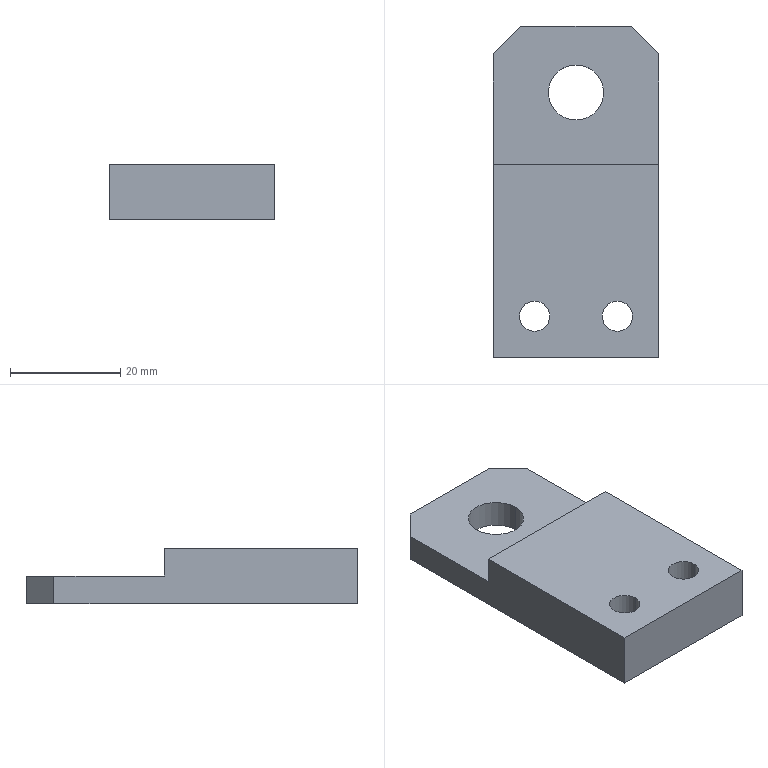Part | STEP file | slingshot displacement cylinder seat | 1 solid | 16 faces | box 30 x 60 x 10 mm | volume 13257 mm3 | plane 10 | cylinder 6 | commonest cylinder face diameters 5.5 x4 10 x2
STEP:
#1=CARTESIAN_POINT('',(0.,0.,0.));
#2=DIRECTION('',(0.,0.,1.));
#3=DIRECTION('',(1.,0.,0.));
#4=AXIS2_PLACEMENT_3D('',#1,#2,#3);
#5=CARTESIAN_POINT('',(-18.899,-2.623,0.));
#6=VERTEX_POINT('',#5);
#7=CARTESIAN_POINT('',(-18.899,-2.623,10.));
#8=VERTEX_POINT('',#7);
#9=CARTESIAN_POINT('',(-18.899,-2.623,0.));
#10=DIRECTION('',(0.,0.,1.));
#11=VECTOR('',#10,1.);
#12=LINE('',#9,#11);
#13=CARTESIAN_POINT('',(-21.649,-2.623,0.));
#14=DIRECTION('',(0.,0.,1.));
#15=DIRECTION('',(1.,0.,0.));
#16=AXIS2_PLACEMENT_3D('',#13,#14,#15);
#17=CYLINDRICAL_SURFACE('',#16,2.75);
#18=CARTESIAN_POINT('',(6.283,0.));
#19=DIRECTION('',(0.,1.));
#20=VECTOR('',#19,1.);
#21=LINE('',#18,#20);
#22=(GEOMETRIC_REPRESENTATION_CONTEXT(2)PARAMETRIC_REPRESENTATION_CONTEXT()REPRESENTATION_CONTEXT('',''));
#23=DEFINITIONAL_REPRESENTATION('',(#21),#22);
#24=PCURVE('',#17,#23);
#25=CARTESIAN_POINT('',(-21.649,-2.623,0.));
#26=DIRECTION('',(0.,0.,1.));
#27=DIRECTION('',(1.,0.,0.));
#28=AXIS2_PLACEMENT_3D('',#25,#26,#27);
#29=CYLINDRICAL_SURFACE('',#28,2.75);
#30=CARTESIAN_POINT('',(0.,0.));
#31=DIRECTION('',(0.,1.));
#32=VECTOR('',#31,1.);
#33=LINE('',#30,#32);
#34=(GEOMETRIC_REPRESENTATION_CONTEXT(2)PARAMETRIC_REPRESENTATION_CONTEXT()REPRESENTATION_CONTEXT('',''));
#35=DEFINITIONAL_REPRESENTATION('',(#33),#34);
#36=PCURVE('',#29,#35);
#37=SURFACE_CURVE('',#12,(#24,#36),.PCURVE_S1.);
#38=EDGE_CURVE('',#6,#8,#37,.T.);
#39=ORIENTED_EDGE('',*,*,#38,.T.);
#40=CARTESIAN_POINT('',(-24.399,-2.623,10.));
#41=VERTEX_POINT('',#40);
#42=CARTESIAN_POINT('',(-21.649,-2.623,10.));
#43=DIRECTION('',(0.,0.,1.));
#44=DIRECTION('',(1.,0.,0.));
#45=AXIS2_PLACEMENT_3D('',#42,#43,#44);
#46=CIRCLE('',#45,2.75);
#47=CARTESIAN_POINT('',(0.,10.));
#48=DIRECTION('',(1.,0.));
#49=VECTOR('',#48,1.);
#50=LINE('',#47,#49);
#51=(GEOMETRIC_REPRESENTATION_CONTEXT(2)PARAMETRIC_REPRESENTATION_CONTEXT()REPRESENTATION_CONTEXT('',''));
#52=DEFINITIONAL_REPRESENTATION('',(#50),#51);
#53=PCURVE('',#17,#52);
#54=CARTESIAN_POINT('',(-29.149,-10.123,10.));
#55=DIRECTION('',(0.,0.,1.));
#56=DIRECTION('',(1.,0.,0.));
#57=AXIS2_PLACEMENT_3D('',#54,#55,#56);
#58=PLANE('',#57);
#59=CARTESIAN_POINT('',(7.5,7.5));
#60=DIRECTION('',(1.,0.));
#61=AXIS2_PLACEMENT_2D('',#59,#60);
#62=CIRCLE('',#61,2.75);
#63=(GEOMETRIC_REPRESENTATION_CONTEXT(2)PARAMETRIC_REPRESENTATION_CONTEXT()REPRESENTATION_CONTEXT('',''));
#64=DEFINITIONAL_REPRESENTATION('',(#62),#63);
#65=PCURVE('',#58,#64);
#66=SURFACE_CURVE('',#46,(#53,#65),.PCURVE_S1.);
#67=EDGE_CURVE('',#41,#8,#66,.T.);
#68=ORIENTED_EDGE('',*,*,#67,.F.);
#69=CARTESIAN_POINT('',(-24.399,-2.623,0.));
#70=VERTEX_POINT('',#69);
#71=CARTESIAN_POINT('',(-24.399,-2.623,0.));
#72=DIRECTION('',(0.,0.,1.));
#73=VECTOR('',#72,1.);
#74=LINE('',#71,#73);
#75=CARTESIAN_POINT('',(3.142,0.));
#76=DIRECTION('',(0.,1.));
#77=VECTOR('',#76,1.);
#78=LINE('',#75,#77);
#79=(GEOMETRIC_REPRESENTATION_CONTEXT(2)PARAMETRIC_REPRESENTATION_CONTEXT()REPRESENTATION_CONTEXT('',''));
#80=DEFINITIONAL_REPRESENTATION('',(#78),#79);
#81=PCURVE('',#17,#80);
#82=CARTESIAN_POINT('',(3.142,0.));
#83=DIRECTION('',(0.,1.));
#84=VECTOR('',#83,1.);
#85=LINE('',#82,#84);
#86=(GEOMETRIC_REPRESENTATION_CONTEXT(2)PARAMETRIC_REPRESENTATION_CONTEXT()REPRESENTATION_CONTEXT('',''));
#87=DEFINITIONAL_REPRESENTATION('',(#85),#86);
#88=PCURVE('',#29,#87);
#89=SURFACE_CURVE('',#74,(#81,#88),.PCURVE_S1.);
#90=EDGE_CURVE('',#70,#41,#89,.T.);
#91=ORIENTED_EDGE('',*,*,#90,.F.);
#92=CARTESIAN_POINT('',(-21.649,-2.623,0.));
#93=DIRECTION('',(0.,0.,1.));
#94=DIRECTION('',(1.,0.,0.));
#95=AXIS2_PLACEMENT_3D('',#92,#93,#94);
#96=CIRCLE('',#95,2.75);
#97=CARTESIAN_POINT('',(0.,0.));
#98=DIRECTION('',(1.,0.));
#99=VECTOR('',#98,1.);
#100=LINE('',#97,#99);
#101=(GEOMETRIC_REPRESENTATION_CONTEXT(2)PARAMETRIC_REPRESENTATION_CONTEXT()REPRESENTATION_CONTEXT('',''));
#102=DEFINITIONAL_REPRESENTATION('',(#100),#101);
#103=PCURVE('',#17,#102);
#104=CARTESIAN_POINT('',(-29.149,-10.123,0.));
#105=DIRECTION('',(0.,0.,1.));
#106=DIRECTION('',(1.,0.,0.));
#107=AXIS2_PLACEMENT_3D('',#104,#105,#106);
#108=PLANE('',#107);
#109=CARTESIAN_POINT('',(7.5,7.5));
#110=DIRECTION('',(1.,0.));
#111=AXIS2_PLACEMENT_2D('',#109,#110);
#112=CIRCLE('',#111,2.75);
#113=(GEOMETRIC_REPRESENTATION_CONTEXT(2)PARAMETRIC_REPRESENTATION_CONTEXT()REPRESENTATION_CONTEXT('',''));
#114=DEFINITIONAL_REPRESENTATION('',(#112),#113);
#115=PCURVE('',#108,#114);
#116=SURFACE_CURVE('',#96,(#103,#115),.PCURVE_S1.);
#117=EDGE_CURVE('',#70,#6,#116,.T.);
#118=ORIENTED_EDGE('',*,*,#117,.T.);
#119=EDGE_LOOP('',(#39,#68,#91,#118));
#120=FACE_BOUND('',#119,.F.);
#121=ADVANCED_FACE('',(#120),#17,.F.);
#122=CARTESIAN_POINT('',(-3.899,-2.623,0.));
#123=VERTEX_POINT('',#122);
#124=CARTESIAN_POINT('',(-3.899,-2.623,10.));
#125=VERTEX_POINT('',#124);
#126=CARTESIAN_POINT('',(-3.899,-2.623,0.));
#127=DIRECTION('',(0.,0.,1.));
#128=VECTOR('',#127,1.);
#129=LINE('',#126,#128);
#130=CARTESIAN_POINT('',(-6.649,-2.623,0.));
#131=DIRECTION('',(0.,0.,1.));
#132=DIRECTION('',(1.,0.,0.));
#133=AXIS2_PLACEMENT_3D('',#130,#131,#132);
#134=CYLINDRICAL_SURFACE('',#133,2.75);
#135=CARTESIAN_POINT('',(6.283,0.));
#136=DIRECTION('',(0.,1.));
#137=VECTOR('',#136,1.);
#138=LINE('',#135,#137);
#139=(GEOMETRIC_REPRESENTATION_CONTEXT(2)PARAMETRIC_REPRESENTATION_CONTEXT()REPRESENTATION_CONTEXT('',''));
#140=DEFINITIONAL_REPRESENTATION('',(#138),#139);
#141=PCURVE('',#134,#140);
#142=CARTESIAN_POINT('',(-6.649,-2.623,0.));
#143=DIRECTION('',(0.,0.,1.));
#144=DIRECTION('',(1.,0.,0.));
#145=AXIS2_PLACEMENT_3D('',#142,#143,#144);
#146=CYLINDRICAL_SURFACE('',#145,2.75);
#147=CARTESIAN_POINT('',(0.,0.));
#148=DIRECTION('',(0.,1.));
#149=VECTOR('',#148,1.);
#150=LINE('',#147,#149);
#151=(GEOMETRIC_REPRESENTATION_CONTEXT(2)PARAMETRIC_REPRESENTATION_CONTEXT()REPRESENTATION_CONTEXT('',''));
#152=DEFINITIONAL_REPRESENTATION('',(#150),#151);
#153=PCURVE('',#146,#152);
#154=SURFACE_CURVE('',#129,(#141,#153),.PCURVE_S1.);
#155=EDGE_CURVE('',#123,#125,#154,.T.);
#156=ORIENTED_EDGE('',*,*,#155,.T.);
#157=CARTESIAN_POINT('',(-9.399,-2.623,10.));
#158=VERTEX_POINT('',#157);
#159=CARTESIAN_POINT('',(-6.649,-2.623,10.));
#160=DIRECTION('',(0.,0.,1.));
#161=DIRECTION('',(1.,0.,0.));
#162=AXIS2_PLACEMENT_3D('',#159,#160,#161);
#163=CIRCLE('',#162,2.75);
#164=CARTESIAN_POINT('',(0.,10.));
#165=DIRECTION('',(1.,0.));
#166=VECTOR('',#165,1.);
#167=LINE('',#164,#166);
#168=(GEOMETRIC_REPRESENTATION_CONTEXT(2)PARAMETRIC_REPRESENTATION_CONTEXT()REPRESENTATION_CONTEXT('',''));
#169=DEFINITIONAL_REPRESENTATION('',(#167),#168);
#170=PCURVE('',#134,#169);
#171=CARTESIAN_POINT('',(22.5,7.5));
#172=DIRECTION('',(1.,0.));
#173=AXIS2_PLACEMENT_2D('',#171,#172);
#174=CIRCLE('',#173,2.75);
#175=(GEOMETRIC_REPRESENTATION_CONTEXT(2)PARAMETRIC_REPRESENTATION_CONTEXT()REPRESENTATION_CONTEXT('',''));
#176=DEFINITIONAL_REPRESENTATION('',(#174),#175);
#177=PCURVE('',#58,#176);
#178=SURFACE_CURVE('',#163,(#170,#177),.PCURVE_S1.);
#179=EDGE_CURVE('',#158,#125,#178,.T.);
#180=ORIENTED_EDGE('',*,*,#179,.F.);
#181=CARTESIAN_POINT('',(-9.399,-2.623,0.));
#182=VERTEX_POINT('',#181);
#183=CARTESIAN_POINT('',(-9.399,-2.623,0.));
#184=DIRECTION('',(0.,0.,1.));
#185=VECTOR('',#184,1.);
#186=LINE('',#183,#185);
#187=CARTESIAN_POINT('',(3.142,0.));
#188=DIRECTION('',(0.,1.));
#189=VECTOR('',#188,1.);
#190=LINE('',#187,#189);
#191=(GEOMETRIC_REPRESENTATION_CONTEXT(2)PARAMETRIC_REPRESENTATION_CONTEXT()REPRESENTATION_CONTEXT('',''));
#192=DEFINITIONAL_REPRESENTATION('',(#190),#191);
#193=PCURVE('',#134,#192);
#194=CARTESIAN_POINT('',(3.142,0.));
#195=DIRECTION('',(0.,1.));
#196=VECTOR('',#195,1.);
#197=LINE('',#194,#196);
#198=(GEOMETRIC_REPRESENTATION_CONTEXT(2)PARAMETRIC_REPRESENTATION_CONTEXT()REPRESENTATION_CONTEXT('',''));
#199=DEFINITIONAL_REPRESENTATION('',(#197),#198);
#200=PCURVE('',#146,#199);
#201=SURFACE_CURVE('',#186,(#193,#200),.PCURVE_S1.);
#202=EDGE_CURVE('',#182,#158,#201,.T.);
#203=ORIENTED_EDGE('',*,*,#202,.F.);
#204=CARTESIAN_POINT('',(-6.649,-2.623,0.));
#205=DIRECTION('',(0.,0.,1.));
#206=DIRECTION('',(1.,0.,0.));
#207=AXIS2_PLACEMENT_3D('',#204,#205,#206);
#208=CIRCLE('',#207,2.75);
#209=CARTESIAN_POINT('',(0.,0.));
#210=DIRECTION('',(1.,0.));
#211=VECTOR('',#210,1.);
#212=LINE('',#209,#211);
#213=(GEOMETRIC_REPRESENTATION_CONTEXT(2)PARAMETRIC_REPRESENTATION_CONTEXT()REPRESENTATION_CONTEXT('',''));
#214=DEFINITIONAL_REPRESENTATION('',(#212),#213);
#215=PCURVE('',#134,#214);
#216=CARTESIAN_POINT('',(22.5,7.5));
#217=DIRECTION('',(1.,0.));
#218=AXIS2_PLACEMENT_2D('',#216,#217);
#219=CIRCLE('',#218,2.75);
#220=(GEOMETRIC_REPRESENTATION_CONTEXT(2)PARAMETRIC_REPRESENTATION_CONTEXT()REPRESENTATION_CONTEXT('',''));
#221=DEFINITIONAL_REPRESENTATION('',(#219),#220);
#222=PCURVE('',#108,#221);
#223=SURFACE_CURVE('',#208,(#215,#222),.PCURVE_S1.);
#224=EDGE_CURVE('',#182,#123,#223,.T.);
#225=ORIENTED_EDGE('',*,*,#224,.T.);
#226=EDGE_LOOP('',(#156,#180,#203,#225));
#227=FACE_BOUND('',#226,.F.);
#228=ADVANCED_FACE('',(#227),#134,.F.);
#229=CARTESIAN_POINT('',(-19.149,37.877,5.));
#230=VERTEX_POINT('',#229);
#231=CARTESIAN_POINT('',(-19.149,37.877,0.));
#232=VERTEX_POINT('',#231);
#233=CARTESIAN_POINT('',(-19.149,37.877,10.));
#234=DIRECTION('',(0.,0.,-1.));
#235=VECTOR('',#234,1.);
#236=LINE('',#233,#235);
#237=CARTESIAN_POINT('',(-14.149,37.877,10.));
#238=DIRECTION('',(0.,0.,-1.));
#239=DIRECTION('',(-1.,0.,0.));
#240=AXIS2_PLACEMENT_3D('',#237,#238,#239);
#241=CYLINDRICAL_SURFACE('',#240,5.);
#242=CARTESIAN_POINT('',(6.283,0.));
#243=DIRECTION('',(0.,1.));
#244=VECTOR('',#243,1.);
#245=LINE('',#242,#244);
#246=(GEOMETRIC_REPRESENTATION_CONTEXT(2)PARAMETRIC_REPRESENTATION_CONTEXT()REPRESENTATION_CONTEXT('',''));
#247=DEFINITIONAL_REPRESENTATION('',(#245),#246);
#248=PCURVE('',#241,#247);
#249=CARTESIAN_POINT('',(-14.149,37.877,10.));
#250=DIRECTION('',(0.,0.,-1.));
#251=DIRECTION('',(-1.,0.,0.));
#252=AXIS2_PLACEMENT_3D('',#249,#250,#251);
#253=CYLINDRICAL_SURFACE('',#252,5.);
#254=CARTESIAN_POINT('',(0.,0.));
#255=DIRECTION('',(0.,1.));
#256=VECTOR('',#255,1.);
#257=LINE('',#254,#256);
#258=(GEOMETRIC_REPRESENTATION_CONTEXT(2)PARAMETRIC_REPRESENTATION_CONTEXT()REPRESENTATION_CONTEXT('',''));
#259=DEFINITIONAL_REPRESENTATION('',(#257),#258);
#260=PCURVE('',#253,#259);
#261=SURFACE_CURVE('',#236,(#248,#260),.PCURVE_S1.);
#262=EDGE_CURVE('',#230,#232,#261,.T.);
#263=ORIENTED_EDGE('',*,*,#262,.T.);
#264=CARTESIAN_POINT('',(-9.149,37.877,0.));
#265=VERTEX_POINT('',#264);
#266=CARTESIAN_POINT('',(-14.149,37.877,0.));
#267=DIRECTION('',(0.,0.,1.));
#268=DIRECTION('',(1.,0.,0.));
#269=AXIS2_PLACEMENT_3D('',#266,#267,#268);
#270=CIRCLE('',#269,5.);
#271=CARTESIAN_POINT('',(9.425,10.));
#272=DIRECTION('',(-1.,0.));
#273=VECTOR('',#272,1.);
#274=LINE('',#271,#273);
#275=(GEOMETRIC_REPRESENTATION_CONTEXT(2)PARAMETRIC_REPRESENTATION_CONTEXT()REPRESENTATION_CONTEXT('',''));
#276=DEFINITIONAL_REPRESENTATION('',(#274),#275);
#277=PCURVE('',#241,#276);
#278=CARTESIAN_POINT('',(15.,48.));
#279=DIRECTION('',(1.,0.));
#280=AXIS2_PLACEMENT_2D('',#278,#279);
#281=CIRCLE('',#280,5.);
#282=(GEOMETRIC_REPRESENTATION_CONTEXT(2)PARAMETRIC_REPRESENTATION_CONTEXT()REPRESENTATION_CONTEXT('',''));
#283=DEFINITIONAL_REPRESENTATION('',(#281),#282);
#284=PCURVE('',#108,#283);
#285=SURFACE_CURVE('',#270,(#277,#284),.PCURVE_S1.);
#286=EDGE_CURVE('',#232,#265,#285,.T.);
#287=ORIENTED_EDGE('',*,*,#286,.T.);
#288=CARTESIAN_POINT('',(-9.149,37.877,5.));
#289=VERTEX_POINT('',#288);
#290=CARTESIAN_POINT('',(-9.149,37.877,10.));
#291=DIRECTION('',(0.,0.,-1.));
#292=VECTOR('',#291,1.);
#293=LINE('',#290,#292);
#294=CARTESIAN_POINT('',(3.142,0.));
#295=DIRECTION('',(0.,1.));
#296=VECTOR('',#295,1.);
#297=LINE('',#294,#296);
#298=(GEOMETRIC_REPRESENTATION_CONTEXT(2)PARAMETRIC_REPRESENTATION_CONTEXT()REPRESENTATION_CONTEXT('',''));
#299=DEFINITIONAL_REPRESENTATION('',(#297),#298);
#300=PCURVE('',#241,#299);
#301=CARTESIAN_POINT('',(3.142,0.));
#302=DIRECTION('',(0.,1.));
#303=VECTOR('',#302,1.);
#304=LINE('',#301,#303);
#305=(GEOMETRIC_REPRESENTATION_CONTEXT(2)PARAMETRIC_REPRESENTATION_CONTEXT()REPRESENTATION_CONTEXT('',''));
#306=DEFINITIONAL_REPRESENTATION('',(#304),#305);
#307=PCURVE('',#253,#306);
#308=SURFACE_CURVE('',#293,(#300,#307),.PCURVE_S1.);
#309=EDGE_CURVE('',#289,#265,#308,.T.);
#310=ORIENTED_EDGE('',*,*,#309,.F.);
#311=CARTESIAN_POINT('',(-14.149,37.877,5.));
#312=DIRECTION('',(0.,0.,1.));
#313=DIRECTION('',(1.,0.,0.));
#314=AXIS2_PLACEMENT_3D('',#311,#312,#313);
#315=CIRCLE('',#314,5.);
#316=CARTESIAN_POINT('',(9.425,5.));
#317=DIRECTION('',(-1.,0.));
#318=VECTOR('',#317,1.);
#319=LINE('',#316,#318);
#320=(GEOMETRIC_REPRESENTATION_CONTEXT(2)PARAMETRIC_REPRESENTATION_CONTEXT()REPRESENTATION_CONTEXT('',''));
#321=DEFINITIONAL_REPRESENTATION('',(#319),#320);
#322=PCURVE('',#241,#321);
#323=CARTESIAN_POINT('',(-36.76,24.877,5.));
#324=DIRECTION('',(0.,0.,1.));
#325=DIRECTION('',(1.,0.,0.));
#326=AXIS2_PLACEMENT_3D('',#323,#324,#325);
#327=PLANE('',#326);
#328=CARTESIAN_POINT('',(22.611,13.));
#329=DIRECTION('',(1.,0.));
#330=AXIS2_PLACEMENT_2D('',#328,#329);
#331=CIRCLE('',#330,5.);
#332=(GEOMETRIC_REPRESENTATION_CONTEXT(2)PARAMETRIC_REPRESENTATION_CONTEXT()REPRESENTATION_CONTEXT('',''));
#333=DEFINITIONAL_REPRESENTATION('',(#331),#332);
#334=PCURVE('',#327,#333);
#335=SURFACE_CURVE('',#315,(#322,#334),.PCURVE_S1.);
#336=EDGE_CURVE('',#230,#289,#335,.T.);
#337=ORIENTED_EDGE('',*,*,#336,.F.);
#338=EDGE_LOOP('',(#263,#287,#310,#337));
#339=FACE_BOUND('',#338,.F.);
#340=ADVANCED_FACE('',(#339),#241,.F.);
#341=CARTESIAN_POINT('',(-4.149,49.877,0.));
#342=VERTEX_POINT('',#341);
#343=CARTESIAN_POINT('',(-24.149,49.877,0.));
#344=VERTEX_POINT('',#343);
#345=CARTESIAN_POINT('',(-29.149,49.877,0.));
#346=DIRECTION('',(-1.,0.,0.));
#347=VECTOR('',#346,1.);
#348=LINE('',#345,#347);
#349=CARTESIAN_POINT('',(-29.149,49.877,10.));
#350=DIRECTION('',(0.,-1.,0.));
#351=DIRECTION('',(0.,0.,-1.));
#352=AXIS2_PLACEMENT_3D('',#349,#350,#351);
#353=PLANE('',#352);
#354=CARTESIAN_POINT('',(10.,0.));
#355=DIRECTION('',(0.,-1.));
#356=VECTOR('',#355,1.);
#357=LINE('',#354,#356);
#358=(GEOMETRIC_REPRESENTATION_CONTEXT(2)PARAMETRIC_REPRESENTATION_CONTEXT()REPRESENTATION_CONTEXT('',''));
#359=DEFINITIONAL_REPRESENTATION('',(#357),#358);
#360=PCURVE('',#353,#359);
#361=CARTESIAN_POINT('',(0.,60.));
#362=DIRECTION('',(-1.,0.));
#363=VECTOR('',#362,1.);
#364=LINE('',#361,#363);
#365=(GEOMETRIC_REPRESENTATION_CONTEXT(2)PARAMETRIC_REPRESENTATION_CONTEXT()REPRESENTATION_CONTEXT('',''));
#366=DEFINITIONAL_REPRESENTATION('',(#364),#365);
#367=PCURVE('',#108,#366);
#368=SURFACE_CURVE('',#348,(#360,#367),.PCURVE_S1.);
#369=EDGE_CURVE('',#342,#344,#368,.T.);
#370=ORIENTED_EDGE('',*,*,#369,.T.);
#371=CARTESIAN_POINT('',(-24.149,49.877,5.));
#372=VERTEX_POINT('',#371);
#373=CARTESIAN_POINT('',(-24.149,49.877,10.));
#374=DIRECTION('',(0.,0.,1.));
#375=VECTOR('',#374,1.);
#376=LINE('',#373,#375);
#377=CARTESIAN_POINT('',(0.,5.));
#378=DIRECTION('',(-1.,0.));
#379=VECTOR('',#378,1.);
#380=LINE('',#377,#379);
#381=(GEOMETRIC_REPRESENTATION_CONTEXT(2)PARAMETRIC_REPRESENTATION_CONTEXT()REPRESENTATION_CONTEXT('',''));
#382=DEFINITIONAL_REPRESENTATION('',(#380),#381);
#383=PCURVE('',#353,#382);
#384=CARTESIAN_POINT('',(-29.149,44.877,10.));
#385=DIRECTION('',(0.7071,-0.7071,0.));
#386=DIRECTION('',(0.7071,0.7071,0.));
#387=AXIS2_PLACEMENT_3D('',#384,#385,#386);
#388=PLANE('',#387);
#389=CARTESIAN_POINT('',(7.071,0.));
#390=DIRECTION('',(0.,1.));
#391=VECTOR('',#390,1.);
#392=LINE('',#389,#391);
#393=(GEOMETRIC_REPRESENTATION_CONTEXT(2)PARAMETRIC_REPRESENTATION_CONTEXT()REPRESENTATION_CONTEXT('',''));
#394=DEFINITIONAL_REPRESENTATION('',(#392),#393);
#395=PCURVE('',#388,#394);
#396=SURFACE_CURVE('',#376,(#383,#395),.PCURVE_S1.);
#397=EDGE_CURVE('',#344,#372,#396,.T.);
#398=ORIENTED_EDGE('',*,*,#397,.T.);
#399=CARTESIAN_POINT('',(-4.149,49.877,5.));
#400=VERTEX_POINT('',#399);
#401=CARTESIAN_POINT('',(-29.149,49.877,5.));
#402=DIRECTION('',(-1.,0.,0.));
#403=VECTOR('',#402,1.);
#404=LINE('',#401,#403);
#405=CARTESIAN_POINT('',(5.,0.));
#406=DIRECTION('',(0.,-1.));
#407=VECTOR('',#406,1.);
#408=LINE('',#405,#407);
#409=(GEOMETRIC_REPRESENTATION_CONTEXT(2)PARAMETRIC_REPRESENTATION_CONTEXT()REPRESENTATION_CONTEXT('',''));
#410=DEFINITIONAL_REPRESENTATION('',(#408),#409);
#411=PCURVE('',#353,#410);
#412=CARTESIAN_POINT('',(7.611,25.));
#413=DIRECTION('',(-1.,0.));
#414=VECTOR('',#413,1.);
#415=LINE('',#412,#414);
#416=(GEOMETRIC_REPRESENTATION_CONTEXT(2)PARAMETRIC_REPRESENTATION_CONTEXT()REPRESENTATION_CONTEXT('',''));
#417=DEFINITIONAL_REPRESENTATION('',(#415),#416);
#418=PCURVE('',#327,#417);
#419=SURFACE_CURVE('',#404,(#411,#418),.PCURVE_S1.);
#420=EDGE_CURVE('',#400,#372,#419,.T.);
#421=ORIENTED_EDGE('',*,*,#420,.F.);
#422=CARTESIAN_POINT('',(-4.149,49.877,10.));
#423=DIRECTION('',(0.,0.,-1.));
#424=VECTOR('',#423,1.);
#425=LINE('',#422,#424);
#426=CARTESIAN_POINT('',(0.,25.));
#427=DIRECTION('',(1.,0.));
#428=VECTOR('',#427,1.);
#429=LINE('',#426,#428);
#430=(GEOMETRIC_REPRESENTATION_CONTEXT(2)PARAMETRIC_REPRESENTATION_CONTEXT()REPRESENTATION_CONTEXT('',''));
#431=DEFINITIONAL_REPRESENTATION('',(#429),#430);
#432=PCURVE('',#353,#431);
#433=CARTESIAN_POINT('',(-4.149,49.877,10.));
#434=DIRECTION('',(-0.7071,-0.7071,0.));
#435=DIRECTION('',(0.7071,-0.7071,0.));
#436=AXIS2_PLACEMENT_3D('',#433,#434,#435);
#437=PLANE('',#436);
#438=CARTESIAN_POINT('',(0.,0.));
#439=DIRECTION('',(0.,-1.));
#440=VECTOR('',#439,1.);
#441=LINE('',#438,#440);
#442=(GEOMETRIC_REPRESENTATION_CONTEXT(2)PARAMETRIC_REPRESENTATION_CONTEXT()REPRESENTATION_CONTEXT('',''));
#443=DEFINITIONAL_REPRESENTATION('',(#441),#442);
#444=PCURVE('',#437,#443);
#445=SURFACE_CURVE('',#425,(#432,#444),.PCURVE_S1.);
#446=EDGE_CURVE('',#400,#342,#445,.T.);
#447=ORIENTED_EDGE('',*,*,#446,.T.);
#448=EDGE_LOOP('',(#370,#398,#421,#447));
#449=FACE_BOUND('',#448,.T.);
#450=ADVANCED_FACE('',(#449),#353,.F.);
#451=CARTESIAN_POINT('',(-14.149,37.877,0.));
#452=DIRECTION('',(0.,0.,1.));
#453=DIRECTION('',(1.,0.,0.));
#454=AXIS2_PLACEMENT_3D('',#451,#452,#453);
#455=CIRCLE('',#454,5.);
#456=CARTESIAN_POINT('',(3.142,10.));
#457=DIRECTION('',(-1.,0.));
#458=VECTOR('',#457,1.);
#459=LINE('',#456,#458);
#460=(GEOMETRIC_REPRESENTATION_CONTEXT(2)PARAMETRIC_REPRESENTATION_CONTEXT()REPRESENTATION_CONTEXT('',''));
#461=DEFINITIONAL_REPRESENTATION('',(#459),#460);
#462=PCURVE('',#253,#461);
#463=CARTESIAN_POINT('',(15.,48.));
#464=DIRECTION('',(1.,0.));
#465=AXIS2_PLACEMENT_2D('',#463,#464);
#466=CIRCLE('',#465,5.);
#467=(GEOMETRIC_REPRESENTATION_CONTEXT(2)PARAMETRIC_REPRESENTATION_CONTEXT()REPRESENTATION_CONTEXT('',''));
#468=DEFINITIONAL_REPRESENTATION('',(#466),#467);
#469=PCURVE('',#108,#468);
#470=SURFACE_CURVE('',#455,(#462,#469),.PCURVE_S1.);
#471=EDGE_CURVE('',#265,#232,#470,.T.);
#472=ORIENTED_EDGE('',*,*,#471,.T.);
#473=ORIENTED_EDGE('',*,*,#262,.F.);
#474=CARTESIAN_POINT('',(-14.149,37.877,5.));
#475=DIRECTION('',(0.,0.,1.));
#476=DIRECTION('',(1.,0.,0.));
#477=AXIS2_PLACEMENT_3D('',#474,#475,#476);
#478=CIRCLE('',#477,5.);
#479=CARTESIAN_POINT('',(3.142,5.));
#480=DIRECTION('',(-1.,0.));
#481=VECTOR('',#480,1.);
#482=LINE('',#479,#481);
#483=(GEOMETRIC_REPRESENTATION_CONTEXT(2)PARAMETRIC_REPRESENTATION_CONTEXT()REPRESENTATION_CONTEXT('',''));
#484=DEFINITIONAL_REPRESENTATION('',(#482),#483);
#485=PCURVE('',#253,#484);
#486=CARTESIAN_POINT('',(22.611,13.));
#487=DIRECTION('',(1.,0.));
#488=AXIS2_PLACEMENT_2D('',#486,#487);
#489=CIRCLE('',#488,5.);
#490=(GEOMETRIC_REPRESENTATION_CONTEXT(2)PARAMETRIC_REPRESENTATION_CONTEXT()REPRESENTATION_CONTEXT('',''));
#491=DEFINITIONAL_REPRESENTATION('',(#489),#490);
#492=PCURVE('',#327,#491);
#493=SURFACE_CURVE('',#478,(#485,#492),.PCURVE_S1.);
#494=EDGE_CURVE('',#289,#230,#493,.T.);
#495=ORIENTED_EDGE('',*,*,#494,.F.);
#496=ORIENTED_EDGE('',*,*,#309,.T.);
#497=EDGE_LOOP('',(#472,#473,#495,#496));
#498=FACE_BOUND('',#497,.F.);
#499=ADVANCED_FACE('',(#498),#253,.F.);
#500=CARTESIAN_POINT('',(-21.649,-2.623,10.));
#501=DIRECTION('',(0.,0.,1.));
#502=DIRECTION('',(1.,0.,0.));
#503=AXIS2_PLACEMENT_3D('',#500,#501,#502);
#504=CIRCLE('',#503,2.75);
#505=CARTESIAN_POINT('',(7.5,7.5));
#506=DIRECTION('',(1.,0.));
#507=AXIS2_PLACEMENT_2D('',#505,#506);
#508=CIRCLE('',#507,2.75);
#509=(GEOMETRIC_REPRESENTATION_CONTEXT(2)PARAMETRIC_REPRESENTATION_CONTEXT()REPRESENTATION_CONTEXT('',''));
#510=DEFINITIONAL_REPRESENTATION('',(#508),#509);
#511=PCURVE('',#58,#510);
#512=CARTESIAN_POINT('',(0.,10.));
#513=DIRECTION('',(1.,0.));
#514=VECTOR('',#513,1.);
#515=LINE('',#512,#514);
#516=(GEOMETRIC_REPRESENTATION_CONTEXT(2)PARAMETRIC_REPRESENTATION_CONTEXT()REPRESENTATION_CONTEXT('',''));
#517=DEFINITIONAL_REPRESENTATION('',(#515),#516);
#518=PCURVE('',#29,#517);
#519=SURFACE_CURVE('',#504,(#511,#518),.PCURVE_S1.);
#520=EDGE_CURVE('',#8,#41,#519,.T.);
#521=ORIENTED_EDGE('',*,*,#520,.F.);
#522=ORIENTED_EDGE('',*,*,#67,.F.);
#523=EDGE_LOOP('',(#521,#522));
#524=FACE_BOUND('',#523,.T.);
#525=CARTESIAN_POINT('',(-6.649,-2.623,10.));
#526=DIRECTION('',(0.,0.,1.));
#527=DIRECTION('',(1.,0.,0.));
#528=AXIS2_PLACEMENT_3D('',#525,#526,#527);
#529=CIRCLE('',#528,2.75);
#530=CARTESIAN_POINT('',(22.5,7.5));
#531=DIRECTION('',(1.,0.));
#532=AXIS2_PLACEMENT_2D('',#530,#531);
#533=CIRCLE('',#532,2.75);
#534=(GEOMETRIC_REPRESENTATION_CONTEXT(2)PARAMETRIC_REPRESENTATION_CONTEXT()REPRESENTATION_CONTEXT('',''));
#535=DEFINITIONAL_REPRESENTATION('',(#533),#534);
#536=PCURVE('',#58,#535);
#537=CARTESIAN_POINT('',(0.,10.));
#538=DIRECTION('',(1.,0.));
#539=VECTOR('',#538,1.);
#540=LINE('',#537,#539);
#541=(GEOMETRIC_REPRESENTATION_CONTEXT(2)PARAMETRIC_REPRESENTATION_CONTEXT()REPRESENTATION_CONTEXT('',''));
#542=DEFINITIONAL_REPRESENTATION('',(#540),#541);
#543=PCURVE('',#146,#542);
#544=SURFACE_CURVE('',#529,(#536,#543),.PCURVE_S1.);
#545=EDGE_CURVE('',#125,#158,#544,.T.);
#546=ORIENTED_EDGE('',*,*,#545,.F.);
#547=ORIENTED_EDGE('',*,*,#179,.F.);
#548=EDGE_LOOP('',(#546,#547));
#549=FACE_BOUND('',#548,.T.);
#550=CARTESIAN_POINT('',(-29.149,24.877,10.));
#551=VERTEX_POINT('',#550);
#552=CARTESIAN_POINT('',(0.8509,24.877,10.));
#553=VERTEX_POINT('',#552);
#554=CARTESIAN_POINT('',(-36.76,24.877,10.));
#555=DIRECTION('',(1.,0.,0.));
#556=VECTOR('',#555,1.);
#557=LINE('',#554,#556);
#558=CARTESIAN_POINT('',(-7.611,35.));
#559=DIRECTION('',(1.,0.));
#560=VECTOR('',#559,1.);
#561=LINE('',#558,#560);
#562=(GEOMETRIC_REPRESENTATION_CONTEXT(2)PARAMETRIC_REPRESENTATION_CONTEXT()REPRESENTATION_CONTEXT('',''));
#563=DEFINITIONAL_REPRESENTATION('',(#561),#562);
#564=PCURVE('',#58,#563);
#565=CARTESIAN_POINT('',(-36.76,24.877,5.));
#566=DIRECTION('',(0.,-1.,0.));
#567=DIRECTION('',(0.,0.,-1.));
#568=AXIS2_PLACEMENT_3D('',#565,#566,#567);
#569=PLANE('',#568);
#570=CARTESIAN_POINT('',(-5.,0.));
#571=DIRECTION('',(0.,1.));
#572=VECTOR('',#571,1.);
#573=LINE('',#570,#572);
#574=(GEOMETRIC_REPRESENTATION_CONTEXT(2)PARAMETRIC_REPRESENTATION_CONTEXT()REPRESENTATION_CONTEXT('',''));
#575=DEFINITIONAL_REPRESENTATION('',(#573),#574);
#576=PCURVE('',#569,#575);
#577=SURFACE_CURVE('',#557,(#564,#576),.PCURVE_S1.);
#578=EDGE_CURVE('',#551,#553,#577,.T.);
#579=ORIENTED_EDGE('',*,*,#578,.F.);
#580=CARTESIAN_POINT('',(-29.149,-10.123,10.));
#581=VERTEX_POINT('',#580);
#582=CARTESIAN_POINT('',(-29.149,49.877,10.));
#583=DIRECTION('',(0.,-1.,0.));
#584=VECTOR('',#583,1.);
#585=LINE('',#582,#584);
#586=CARTESIAN_POINT('',(0.,60.));
#587=DIRECTION('',(0.,-1.));
#588=VECTOR('',#587,1.);
#589=LINE('',#586,#588);
#590=(GEOMETRIC_REPRESENTATION_CONTEXT(2)PARAMETRIC_REPRESENTATION_CONTEXT()REPRESENTATION_CONTEXT('',''));
#591=DEFINITIONAL_REPRESENTATION('',(#589),#590);
#592=PCURVE('',#58,#591);
#593=CARTESIAN_POINT('',(-29.149,49.877,10.));
#594=DIRECTION('',(1.,0.,0.));
#595=DIRECTION('',(0.,1.,0.));
#596=AXIS2_PLACEMENT_3D('',#593,#594,#595);
#597=PLANE('',#596);
#598=CARTESIAN_POINT('',(0.,0.));
#599=DIRECTION('',(-1.,0.));
#600=VECTOR('',#599,1.);
#601=LINE('',#598,#600);
#602=(GEOMETRIC_REPRESENTATION_CONTEXT(2)PARAMETRIC_REPRESENTATION_CONTEXT()REPRESENTATION_CONTEXT('',''));
#603=DEFINITIONAL_REPRESENTATION('',(#601),#602);
#604=PCURVE('',#597,#603);
#605=SURFACE_CURVE('',#585,(#592,#604),.PCURVE_S1.);
#606=EDGE_CURVE('',#551,#581,#605,.T.);
#607=ORIENTED_EDGE('',*,*,#606,.T.);
#608=CARTESIAN_POINT('',(0.8509,-10.123,10.));
#609=VERTEX_POINT('',#608);
#610=CARTESIAN_POINT('',(-29.149,-10.123,10.));
#611=DIRECTION('',(1.,0.,0.));
#612=VECTOR('',#611,1.);
#613=LINE('',#610,#612);
#614=CARTESIAN_POINT('',(0.,0.));
#615=DIRECTION('',(1.,0.));
#616=VECTOR('',#615,1.);
#617=LINE('',#614,#616);
#618=(GEOMETRIC_REPRESENTATION_CONTEXT(2)PARAMETRIC_REPRESENTATION_CONTEXT()REPRESENTATION_CONTEXT('',''));
#619=DEFINITIONAL_REPRESENTATION('',(#617),#618);
#620=PCURVE('',#58,#619);
#621=CARTESIAN_POINT('',(-29.149,-10.123,10.));
#622=DIRECTION('',(0.,1.,0.));
#623=DIRECTION('',(0.,0.,1.));
#624=AXIS2_PLACEMENT_3D('',#621,#622,#623);
#625=PLANE('',#624);
#626=CARTESIAN_POINT('',(0.,0.));
#627=DIRECTION('',(0.,1.));
#628=VECTOR('',#627,1.);
#629=LINE('',#626,#628);
#630=(GEOMETRIC_REPRESENTATION_CONTEXT(2)PARAMETRIC_REPRESENTATION_CONTEXT()REPRESENTATION_CONTEXT('',''));
#631=DEFINITIONAL_REPRESENTATION('',(#629),#630);
#632=PCURVE('',#625,#631);
#633=SURFACE_CURVE('',#613,(#620,#632),.PCURVE_S1.);
#634=EDGE_CURVE('',#581,#609,#633,.T.);
#635=ORIENTED_EDGE('',*,*,#634,.T.);
#636=CARTESIAN_POINT('',(0.8509,49.877,10.));
#637=DIRECTION('',(0.,1.,0.));
#638=VECTOR('',#637,1.);
#639=LINE('',#636,#638);
#640=CARTESIAN_POINT('',(30.,60.));
#641=DIRECTION('',(0.,1.));
#642=VECTOR('',#641,1.);
#643=LINE('',#640,#642);
#644=(GEOMETRIC_REPRESENTATION_CONTEXT(2)PARAMETRIC_REPRESENTATION_CONTEXT()REPRESENTATION_CONTEXT('',''));
#645=DEFINITIONAL_REPRESENTATION('',(#643),#644);
#646=PCURVE('',#58,#645);
#647=CARTESIAN_POINT('',(0.8509,49.877,10.));
#648=DIRECTION('',(-1.,0.,0.));
#649=DIRECTION('',(0.,-1.,0.));
#650=AXIS2_PLACEMENT_3D('',#647,#648,#649);
#651=PLANE('',#650);
#652=CARTESIAN_POINT('',(0.,0.));
#653=DIRECTION('',(-1.,0.));
#654=VECTOR('',#653,1.);
#655=LINE('',#652,#654);
#656=(GEOMETRIC_REPRESENTATION_CONTEXT(2)PARAMETRIC_REPRESENTATION_CONTEXT()REPRESENTATION_CONTEXT('',''));
#657=DEFINITIONAL_REPRESENTATION('',(#655),#656);
#658=PCURVE('',#651,#657);
#659=SURFACE_CURVE('',#639,(#646,#658),.PCURVE_S1.);
#660=EDGE_CURVE('',#609,#553,#659,.T.);
#661=ORIENTED_EDGE('',*,*,#660,.T.);
#662=EDGE_LOOP('',(#579,#607,#635,#661));
#663=FACE_BOUND('',#662,.T.);
#664=ADVANCED_FACE('',(#524,#549,#663),#58,.T.);
#665=CARTESIAN_POINT('',(-21.649,-2.623,0.));
#666=DIRECTION('',(0.,0.,1.));
#667=DIRECTION('',(1.,0.,0.));
#668=AXIS2_PLACEMENT_3D('',#665,#666,#667);
#669=CIRCLE('',#668,2.75);
#670=CARTESIAN_POINT('',(7.5,7.5));
#671=DIRECTION('',(1.,0.));
#672=AXIS2_PLACEMENT_2D('',#670,#671);
#673=CIRCLE('',#672,2.75);
#674=(GEOMETRIC_REPRESENTATION_CONTEXT(2)PARAMETRIC_REPRESENTATION_CONTEXT()REPRESENTATION_CONTEXT('',''));
#675=DEFINITIONAL_REPRESENTATION('',(#673),#674);
#676=PCURVE('',#108,#675);
#677=CARTESIAN_POINT('',(0.,0.));
#678=DIRECTION('',(1.,0.));
#679=VECTOR('',#678,1.);
#680=LINE('',#677,#679);
#681=(GEOMETRIC_REPRESENTATION_CONTEXT(2)PARAMETRIC_REPRESENTATION_CONTEXT()REPRESENTATION_CONTEXT('',''));
#682=DEFINITIONAL_REPRESENTATION('',(#680),#681);
#683=PCURVE('',#29,#682);
#684=SURFACE_CURVE('',#669,(#676,#683),.PCURVE_S1.);
#685=EDGE_CURVE('',#6,#70,#684,.T.);
#686=ORIENTED_EDGE('',*,*,#685,.T.);
#687=ORIENTED_EDGE('',*,*,#117,.T.);
#688=EDGE_LOOP('',(#686,#687));
#689=FACE_BOUND('',#688,.T.);
#690=CARTESIAN_POINT('',(-6.649,-2.623,0.));
#691=DIRECTION('',(0.,0.,1.));
#692=DIRECTION('',(1.,0.,0.));
#693=AXIS2_PLACEMENT_3D('',#690,#691,#692);
#694=CIRCLE('',#693,2.75);
#695=CARTESIAN_POINT('',(22.5,7.5));
#696=DIRECTION('',(1.,0.));
#697=AXIS2_PLACEMENT_2D('',#695,#696);
#698=CIRCLE('',#697,2.75);
#699=(GEOMETRIC_REPRESENTATION_CONTEXT(2)PARAMETRIC_REPRESENTATION_CONTEXT()REPRESENTATION_CONTEXT('',''));
#700=DEFINITIONAL_REPRESENTATION('',(#698),#699);
#701=PCURVE('',#108,#700);
#702=CARTESIAN_POINT('',(0.,0.));
#703=DIRECTION('',(1.,0.));
#704=VECTOR('',#703,1.);
#705=LINE('',#702,#704);
#706=(GEOMETRIC_REPRESENTATION_CONTEXT(2)PARAMETRIC_REPRESENTATION_CONTEXT()REPRESENTATION_CONTEXT('',''));
#707=DEFINITIONAL_REPRESENTATION('',(#705),#706);
#708=PCURVE('',#146,#707);
#709=SURFACE_CURVE('',#694,(#701,#708),.PCURVE_S1.);
#710=EDGE_CURVE('',#123,#182,#709,.T.);
#711=ORIENTED_EDGE('',*,*,#710,.T.);
#712=ORIENTED_EDGE('',*,*,#224,.T.);
#713=EDGE_LOOP('',(#711,#712));
#714=FACE_BOUND('',#713,.T.);
#715=CARTESIAN_POINT('',(-29.149,44.877,0.));
#716=VERTEX_POINT('',#715);
#717=CARTESIAN_POINT('',(-29.149,-10.123,0.));
#718=VERTEX_POINT('',#717);
#719=CARTESIAN_POINT('',(-29.149,49.877,0.));
#720=DIRECTION('',(0.,-1.,0.));
#721=VECTOR('',#720,1.);
#722=LINE('',#719,#721);
#723=CARTESIAN_POINT('',(0.,60.));
#724=DIRECTION('',(0.,-1.));
#725=VECTOR('',#724,1.);
#726=LINE('',#723,#725);
#727=(GEOMETRIC_REPRESENTATION_CONTEXT(2)PARAMETRIC_REPRESENTATION_CONTEXT()REPRESENTATION_CONTEXT('',''));
#728=DEFINITIONAL_REPRESENTATION('',(#726),#727);
#729=PCURVE('',#108,#728);
#730=CARTESIAN_POINT('',(0.,-10.));
#731=DIRECTION('',(-1.,0.));
#732=VECTOR('',#731,1.);
#733=LINE('',#730,#732);
#734=(GEOMETRIC_REPRESENTATION_CONTEXT(2)PARAMETRIC_REPRESENTATION_CONTEXT()REPRESENTATION_CONTEXT('',''));
#735=DEFINITIONAL_REPRESENTATION('',(#733),#734);
#736=PCURVE('',#597,#735);
#737=SURFACE_CURVE('',#722,(#729,#736),.PCURVE_S1.);
#738=EDGE_CURVE('',#716,#718,#737,.T.);
#739=ORIENTED_EDGE('',*,*,#738,.F.);
#740=CARTESIAN_POINT('',(-29.149,44.877,0.));
#741=DIRECTION('',(0.7071,0.7071,0.));
#742=VECTOR('',#741,1.);
#743=LINE('',#740,#742);
#744=CARTESIAN_POINT('',(0.,55.));
#745=DIRECTION('',(0.7071,0.7071));
#746=VECTOR('',#745,1.);
#747=LINE('',#744,#746);
#748=(GEOMETRIC_REPRESENTATION_CONTEXT(2)PARAMETRIC_REPRESENTATION_CONTEXT()REPRESENTATION_CONTEXT('',''));
#749=DEFINITIONAL_REPRESENTATION('',(#747),#748);
#750=PCURVE('',#108,#749);
#751=CARTESIAN_POINT('',(0.,-10.));
#752=DIRECTION('',(1.,0.));
#753=VECTOR('',#752,1.);
#754=LINE('',#751,#753);
#755=(GEOMETRIC_REPRESENTATION_CONTEXT(2)PARAMETRIC_REPRESENTATION_CONTEXT()REPRESENTATION_CONTEXT('',''));
#756=DEFINITIONAL_REPRESENTATION('',(#754),#755);
#757=PCURVE('',#388,#756);
#758=SURFACE_CURVE('',#743,(#750,#757),.PCURVE_S1.);
#759=EDGE_CURVE('',#716,#344,#758,.T.);
#760=ORIENTED_EDGE('',*,*,#759,.T.);
#761=ORIENTED_EDGE('',*,*,#369,.F.);
#762=CARTESIAN_POINT('',(0.8509,44.877,0.));
#763=VERTEX_POINT('',#762);
#764=CARTESIAN_POINT('',(-4.149,49.877,0.));
#765=DIRECTION('',(0.7071,-0.7071,0.));
#766=VECTOR('',#765,1.);
#767=LINE('',#764,#766);
#768=CARTESIAN_POINT('',(25.,60.));
#769=DIRECTION('',(0.7071,-0.7071));
#770=VECTOR('',#769,1.);
#771=LINE('',#768,#770);
#772=(GEOMETRIC_REPRESENTATION_CONTEXT(2)PARAMETRIC_REPRESENTATION_CONTEXT()REPRESENTATION_CONTEXT('',''));
#773=DEFINITIONAL_REPRESENTATION('',(#771),#772);
#774=PCURVE('',#108,#773);
#775=CARTESIAN_POINT('',(0.,-10.));
#776=DIRECTION('',(1.,0.));
#777=VECTOR('',#776,1.);
#778=LINE('',#775,#777);
#779=(GEOMETRIC_REPRESENTATION_CONTEXT(2)PARAMETRIC_REPRESENTATION_CONTEXT()REPRESENTATION_CONTEXT('',''));
#780=DEFINITIONAL_REPRESENTATION('',(#778),#779);
#781=PCURVE('',#437,#780);
#782=SURFACE_CURVE('',#767,(#774,#781),.PCURVE_S1.);
#783=EDGE_CURVE('',#342,#763,#782,.T.);
#784=ORIENTED_EDGE('',*,*,#783,.T.);
#785=CARTESIAN_POINT('',(0.8509,-10.123,0.));
#786=VERTEX_POINT('',#785);
#787=CARTESIAN_POINT('',(0.8509,49.877,0.));
#788=DIRECTION('',(0.,1.,0.));
#789=VECTOR('',#788,1.);
#790=LINE('',#787,#789);
#791=CARTESIAN_POINT('',(30.,60.));
#792=DIRECTION('',(0.,1.));
#793=VECTOR('',#792,1.);
#794=LINE('',#791,#793);
#795=(GEOMETRIC_REPRESENTATION_CONTEXT(2)PARAMETRIC_REPRESENTATION_CONTEXT()REPRESENTATION_CONTEXT('',''));
#796=DEFINITIONAL_REPRESENTATION('',(#794),#795);
#797=PCURVE('',#108,#796);
#798=CARTESIAN_POINT('',(0.,-10.));
#799=DIRECTION('',(-1.,0.));
#800=VECTOR('',#799,1.);
#801=LINE('',#798,#800);
#802=(GEOMETRIC_REPRESENTATION_CONTEXT(2)PARAMETRIC_REPRESENTATION_CONTEXT()REPRESENTATION_CONTEXT('',''));
#803=DEFINITIONAL_REPRESENTATION('',(#801),#802);
#804=PCURVE('',#651,#803);
#805=SURFACE_CURVE('',#790,(#797,#804),.PCURVE_S1.);
#806=EDGE_CURVE('',#786,#763,#805,.T.);
#807=ORIENTED_EDGE('',*,*,#806,.F.);
#808=CARTESIAN_POINT('',(-29.149,-10.123,0.));
#809=DIRECTION('',(1.,0.,0.));
#810=VECTOR('',#809,1.);
#811=LINE('',#808,#810);
#812=CARTESIAN_POINT('',(0.,0.));
#813=DIRECTION('',(1.,0.));
#814=VECTOR('',#813,1.);
#815=LINE('',#812,#814);
#816=(GEOMETRIC_REPRESENTATION_CONTEXT(2)PARAMETRIC_REPRESENTATION_CONTEXT()REPRESENTATION_CONTEXT('',''));
#817=DEFINITIONAL_REPRESENTATION('',(#815),#816);
#818=PCURVE('',#108,#817);
#819=CARTESIAN_POINT('',(-10.,0.));
#820=DIRECTION('',(0.,1.));
#821=VECTOR('',#820,1.);
#822=LINE('',#819,#821);
#823=(GEOMETRIC_REPRESENTATION_CONTEXT(2)PARAMETRIC_REPRESENTATION_CONTEXT()REPRESENTATION_CONTEXT('',''));
#824=DEFINITIONAL_REPRESENTATION('',(#822),#823);
#825=PCURVE('',#625,#824);
#826=SURFACE_CURVE('',#811,(#818,#825),.PCURVE_S1.);
#827=EDGE_CURVE('',#718,#786,#826,.T.);
#828=ORIENTED_EDGE('',*,*,#827,.F.);
#829=EDGE_LOOP('',(#739,#760,#761,#784,#807,#828));
#830=FACE_BOUND('',#829,.T.);
#831=ORIENTED_EDGE('',*,*,#286,.T.);
#832=ORIENTED_EDGE('',*,*,#471,.T.);
#833=EDGE_LOOP('',(#831,#832));
#834=FACE_BOUND('',#833,.T.);
#835=ADVANCED_FACE('',(#689,#714,#830,#834),#108,.F.);
#836=CARTESIAN_POINT('',(-29.149,44.877,5.));
#837=VERTEX_POINT('',#836);
#838=CARTESIAN_POINT('',(-29.149,24.877,5.));
#839=VERTEX_POINT('',#838);
#840=CARTESIAN_POINT('',(-29.149,49.877,5.));
#841=DIRECTION('',(0.,-1.,0.));
#842=VECTOR('',#841,1.);
#843=LINE('',#840,#842);
#844=CARTESIAN_POINT('',(0.,-5.));
#845=DIRECTION('',(-1.,0.));
#846=VECTOR('',#845,1.);
#847=LINE('',#844,#846);
#848=(GEOMETRIC_REPRESENTATION_CONTEXT(2)PARAMETRIC_REPRESENTATION_CONTEXT()REPRESENTATION_CONTEXT('',''));
#849=DEFINITIONAL_REPRESENTATION('',(#847),#848);
#850=PCURVE('',#597,#849);
#851=CARTESIAN_POINT('',(7.611,25.));
#852=DIRECTION('',(0.,-1.));
#853=VECTOR('',#852,1.);
#854=LINE('',#851,#853);
#855=(GEOMETRIC_REPRESENTATION_CONTEXT(2)PARAMETRIC_REPRESENTATION_CONTEXT()REPRESENTATION_CONTEXT('',''));
#856=DEFINITIONAL_REPRESENTATION('',(#854),#855);
#857=PCURVE('',#327,#856);
#858=SURFACE_CURVE('',#843,(#850,#857),.PCURVE_S1.);
#859=EDGE_CURVE('',#837,#839,#858,.T.);
#860=ORIENTED_EDGE('',*,*,#859,.F.);
#861=CARTESIAN_POINT('',(-29.149,44.877,10.));
#862=DIRECTION('',(0.,0.,-1.));
#863=VECTOR('',#862,1.);
#864=LINE('',#861,#863);
#865=CARTESIAN_POINT('',(-5.,0.));
#866=DIRECTION('',(0.,-1.));
#867=VECTOR('',#866,1.);
#868=LINE('',#865,#867);
#869=(GEOMETRIC_REPRESENTATION_CONTEXT(2)PARAMETRIC_REPRESENTATION_CONTEXT()REPRESENTATION_CONTEXT('',''));
#870=DEFINITIONAL_REPRESENTATION('',(#868),#869);
#871=PCURVE('',#597,#870);
#872=CARTESIAN_POINT('',(0.,0.));
#873=DIRECTION('',(0.,-1.));
#874=VECTOR('',#873,1.);
#875=LINE('',#872,#874);
#876=(GEOMETRIC_REPRESENTATION_CONTEXT(2)PARAMETRIC_REPRESENTATION_CONTEXT()REPRESENTATION_CONTEXT('',''));
#877=DEFINITIONAL_REPRESENTATION('',(#875),#876);
#878=PCURVE('',#388,#877);
#879=SURFACE_CURVE('',#864,(#871,#878),.PCURVE_S1.);
#880=EDGE_CURVE('',#837,#716,#879,.T.);
#881=ORIENTED_EDGE('',*,*,#880,.T.);
#882=ORIENTED_EDGE('',*,*,#738,.T.);
#883=CARTESIAN_POINT('',(-29.149,-10.123,10.));
#884=DIRECTION('',(0.,0.,-1.));
#885=VECTOR('',#884,1.);
#886=LINE('',#883,#885);
#887=CARTESIAN_POINT('',(-60.,0.));
#888=DIRECTION('',(0.,-1.));
#889=VECTOR('',#888,1.);
#890=LINE('',#887,#889);
#891=(GEOMETRIC_REPRESENTATION_CONTEXT(2)PARAMETRIC_REPRESENTATION_CONTEXT()REPRESENTATION_CONTEXT('',''));
#892=DEFINITIONAL_REPRESENTATION('',(#890),#891);
#893=PCURVE('',#597,#892);
#894=CARTESIAN_POINT('',(0.,0.));
#895=DIRECTION('',(-1.,0.));
#896=VECTOR('',#895,1.);
#897=LINE('',#894,#896);
#898=(GEOMETRIC_REPRESENTATION_CONTEXT(2)PARAMETRIC_REPRESENTATION_CONTEXT()REPRESENTATION_CONTEXT('',''));
#899=DEFINITIONAL_REPRESENTATION('',(#897),#898);
#900=PCURVE('',#625,#899);
#901=SURFACE_CURVE('',#886,(#893,#900),.PCURVE_S1.);
#902=EDGE_CURVE('',#581,#718,#901,.T.);
#903=ORIENTED_EDGE('',*,*,#902,.F.);
#904=ORIENTED_EDGE('',*,*,#606,.F.);
#905=CARTESIAN_POINT('',(-29.149,24.877,10.));
#906=DIRECTION('',(0.,0.,-1.));
#907=VECTOR('',#906,1.);
#908=LINE('',#905,#907);
#909=CARTESIAN_POINT('',(-25.,0.));
#910=DIRECTION('',(0.,-1.));
#911=VECTOR('',#910,1.);
#912=LINE('',#909,#911);
#913=(GEOMETRIC_REPRESENTATION_CONTEXT(2)PARAMETRIC_REPRESENTATION_CONTEXT()REPRESENTATION_CONTEXT('',''));
#914=DEFINITIONAL_REPRESENTATION('',(#912),#913);
#915=PCURVE('',#597,#914);
#916=CARTESIAN_POINT('',(-5.,7.611));
#917=DIRECTION('',(1.,0.));
#918=VECTOR('',#917,1.);
#919=LINE('',#916,#918);
#920=(GEOMETRIC_REPRESENTATION_CONTEXT(2)PARAMETRIC_REPRESENTATION_CONTEXT()REPRESENTATION_CONTEXT('',''));
#921=DEFINITIONAL_REPRESENTATION('',(#919),#920);
#922=PCURVE('',#569,#921);
#923=SURFACE_CURVE('',#908,(#915,#922),.PCURVE_S1.);
#924=EDGE_CURVE('',#551,#839,#923,.T.);
#925=ORIENTED_EDGE('',*,*,#924,.T.);
#926=EDGE_LOOP('',(#860,#881,#882,#903,#904,#925));
#927=FACE_BOUND('',#926,.T.);
#928=ADVANCED_FACE('',(#927),#597,.F.);
#929=ORIENTED_EDGE('',*,*,#827,.T.);
#930=CARTESIAN_POINT('',(0.8509,-10.123,10.));
#931=DIRECTION('',(0.,0.,-1.));
#932=VECTOR('',#931,1.);
#933=LINE('',#930,#932);
#934=CARTESIAN_POINT('',(0.,30.));
#935=DIRECTION('',(-1.,0.));
#936=VECTOR('',#935,1.);
#937=LINE('',#934,#936);
#938=(GEOMETRIC_REPRESENTATION_CONTEXT(2)PARAMETRIC_REPRESENTATION_CONTEXT()REPRESENTATION_CONTEXT('',''));
#939=DEFINITIONAL_REPRESENTATION('',(#937),#938);
#940=PCURVE('',#625,#939);
#941=CARTESIAN_POINT('',(60.,0.));
#942=DIRECTION('',(0.,-1.));
#943=VECTOR('',#942,1.);
#944=LINE('',#941,#943);
#945=(GEOMETRIC_REPRESENTATION_CONTEXT(2)PARAMETRIC_REPRESENTATION_CONTEXT()REPRESENTATION_CONTEXT('',''));
#946=DEFINITIONAL_REPRESENTATION('',(#944),#945);
#947=PCURVE('',#651,#946);
#948=SURFACE_CURVE('',#933,(#940,#947),.PCURVE_S1.);
#949=EDGE_CURVE('',#609,#786,#948,.T.);
#950=ORIENTED_EDGE('',*,*,#949,.F.);
#951=ORIENTED_EDGE('',*,*,#634,.F.);
#952=ORIENTED_EDGE('',*,*,#902,.T.);
#953=EDGE_LOOP('',(#929,#950,#951,#952));
#954=FACE_BOUND('',#953,.T.);
#955=ADVANCED_FACE('',(#954),#625,.F.);
#956=ORIENTED_EDGE('',*,*,#806,.T.);
#957=CARTESIAN_POINT('',(0.8509,44.877,5.));
#958=VERTEX_POINT('',#957);
#959=CARTESIAN_POINT('',(0.8509,44.877,10.));
#960=DIRECTION('',(0.,0.,1.));
#961=VECTOR('',#960,1.);
#962=LINE('',#959,#961);
#963=CARTESIAN_POINT('',(5.,0.));
#964=DIRECTION('',(0.,1.));
#965=VECTOR('',#964,1.);
#966=LINE('',#963,#965);
#967=(GEOMETRIC_REPRESENTATION_CONTEXT(2)PARAMETRIC_REPRESENTATION_CONTEXT()REPRESENTATION_CONTEXT('',''));
#968=DEFINITIONAL_REPRESENTATION('',(#966),#967);
#969=PCURVE('',#651,#968);
#970=CARTESIAN_POINT('',(7.071,0.));
#971=DIRECTION('',(0.,1.));
#972=VECTOR('',#971,1.);
#973=LINE('',#970,#972);
#974=(GEOMETRIC_REPRESENTATION_CONTEXT(2)PARAMETRIC_REPRESENTATION_CONTEXT()REPRESENTATION_CONTEXT('',''));
#975=DEFINITIONAL_REPRESENTATION('',(#973),#974);
#976=PCURVE('',#437,#975);
#977=SURFACE_CURVE('',#962,(#969,#976),.PCURVE_S1.);
#978=EDGE_CURVE('',#763,#958,#977,.T.);
#979=ORIENTED_EDGE('',*,*,#978,.T.);
#980=CARTESIAN_POINT('',(0.8509,24.877,5.));
#981=VERTEX_POINT('',#980);
#982=CARTESIAN_POINT('',(0.8509,49.877,5.));
#983=DIRECTION('',(0.,1.,0.));
#984=VECTOR('',#983,1.);
#985=LINE('',#982,#984);
#986=CARTESIAN_POINT('',(0.,-5.));
#987=DIRECTION('',(-1.,0.));
#988=VECTOR('',#987,1.);
#989=LINE('',#986,#988);
#990=(GEOMETRIC_REPRESENTATION_CONTEXT(2)PARAMETRIC_REPRESENTATION_CONTEXT()REPRESENTATION_CONTEXT('',''));
#991=DEFINITIONAL_REPRESENTATION('',(#989),#990);
#992=PCURVE('',#651,#991);
#993=CARTESIAN_POINT('',(37.611,25.));
#994=DIRECTION('',(0.,1.));
#995=VECTOR('',#994,1.);
#996=LINE('',#993,#995);
#997=(GEOMETRIC_REPRESENTATION_CONTEXT(2)PARAMETRIC_REPRESENTATION_CONTEXT()REPRESENTATION_CONTEXT('',''));
#998=DEFINITIONAL_REPRESENTATION('',(#996),#997);
#999=PCURVE('',#327,#998);
#1000=SURFACE_CURVE('',#985,(#992,#999),.PCURVE_S1.);
#1001=EDGE_CURVE('',#981,#958,#1000,.T.);
#1002=ORIENTED_EDGE('',*,*,#1001,.F.);
#1003=CARTESIAN_POINT('',(0.8509,24.877,10.));
#1004=DIRECTION('',(0.,0.,1.));
#1005=VECTOR('',#1004,1.);
#1006=LINE('',#1003,#1005);
#1007=CARTESIAN_POINT('',(25.,0.));
#1008=DIRECTION('',(0.,1.));
#1009=VECTOR('',#1008,1.);
#1010=LINE('',#1007,#1009);
#1011=(GEOMETRIC_REPRESENTATION_CONTEXT(2)PARAMETRIC_REPRESENTATION_CONTEXT()REPRESENTATION_CONTEXT('',''));
#1012=DEFINITIONAL_REPRESENTATION('',(#1010),#1011);
#1013=PCURVE('',#651,#1012);
#1014=CARTESIAN_POINT('',(-5.,37.611));
#1015=DIRECTION('',(-1.,0.));
#1016=VECTOR('',#1015,1.);
#1017=LINE('',#1014,#1016);
#1018=(GEOMETRIC_REPRESENTATION_CONTEXT(2)PARAMETRIC_REPRESENTATION_CONTEXT()REPRESENTATION_CONTEXT('',''));
#1019=DEFINITIONAL_REPRESENTATION('',(#1017),#1018);
#1020=PCURVE('',#569,#1019);
#1021=SURFACE_CURVE('',#1006,(#1013,#1020),.PCURVE_S1.);
#1022=EDGE_CURVE('',#981,#553,#1021,.T.);
#1023=ORIENTED_EDGE('',*,*,#1022,.T.);
#1024=ORIENTED_EDGE('',*,*,#660,.F.);
#1025=ORIENTED_EDGE('',*,*,#949,.T.);
#1026=EDGE_LOOP('',(#956,#979,#1002,#1023,#1024,#1025));
#1027=FACE_BOUND('',#1026,.T.);
#1028=ADVANCED_FACE('',(#1027),#651,.F.);
#1029=ORIENTED_EDGE('',*,*,#578,.T.);
#1030=ORIENTED_EDGE('',*,*,#1022,.F.);
#1031=CARTESIAN_POINT('',(-36.76,24.877,5.));
#1032=DIRECTION('',(1.,0.,0.));
#1033=VECTOR('',#1032,1.);
#1034=LINE('',#1031,#1033);
#1035=CARTESIAN_POINT('',(0.,0.));
#1036=DIRECTION('',(0.,1.));
#1037=VECTOR('',#1036,1.);
#1038=LINE('',#1035,#1037);
#1039=(GEOMETRIC_REPRESENTATION_CONTEXT(2)PARAMETRIC_REPRESENTATION_CONTEXT()REPRESENTATION_CONTEXT('',''));
#1040=DEFINITIONAL_REPRESENTATION('',(#1038),#1039);
#1041=PCURVE('',#569,#1040);
#1042=CARTESIAN_POINT('',(0.,0.));
#1043=DIRECTION('',(1.,0.));
#1044=VECTOR('',#1043,1.);
#1045=LINE('',#1042,#1044);
#1046=(GEOMETRIC_REPRESENTATION_CONTEXT(2)PARAMETRIC_REPRESENTATION_CONTEXT()REPRESENTATION_CONTEXT('',''));
#1047=DEFINITIONAL_REPRESENTATION('',(#1045),#1046);
#1048=PCURVE('',#327,#1047);
#1049=SURFACE_CURVE('',#1034,(#1041,#1048),.PCURVE_S1.);
#1050=EDGE_CURVE('',#839,#981,#1049,.T.);
#1051=ORIENTED_EDGE('',*,*,#1050,.F.);
#1052=ORIENTED_EDGE('',*,*,#924,.F.);
#1053=EDGE_LOOP('',(#1029,#1030,#1051,#1052));
#1054=FACE_BOUND('',#1053,.T.);
#1055=ADVANCED_FACE('',(#1054),#569,.F.);
#1056=ORIENTED_EDGE('',*,*,#336,.F.);
#1057=ORIENTED_EDGE('',*,*,#494,.F.);
#1058=EDGE_LOOP('',(#1056,#1057));
#1059=FACE_BOUND('',#1058,.T.);
#1060=ORIENTED_EDGE('',*,*,#420,.T.);
#1061=CARTESIAN_POINT('',(-42.955,31.072,5.));
#1062=DIRECTION('',(-0.7071,-0.7071,0.));
#1063=VECTOR('',#1062,1.);
#1064=LINE('',#1061,#1063);
#1065=CARTESIAN_POINT('',(-6.194,6.194));
#1066=DIRECTION('',(-0.7071,-0.7071));
#1067=VECTOR('',#1066,1.);
#1068=LINE('',#1065,#1067);
#1069=(GEOMETRIC_REPRESENTATION_CONTEXT(2)PARAMETRIC_REPRESENTATION_CONTEXT()REPRESENTATION_CONTEXT('',''));
#1070=DEFINITIONAL_REPRESENTATION('',(#1068),#1069);
#1071=PCURVE('',#327,#1070);
#1072=CARTESIAN_POINT('',(-19.524,-5.));
#1073=DIRECTION('',(-1.,0.));
#1074=VECTOR('',#1073,1.);
#1075=LINE('',#1072,#1074);
#1076=(GEOMETRIC_REPRESENTATION_CONTEXT(2)PARAMETRIC_REPRESENTATION_CONTEXT()REPRESENTATION_CONTEXT('',''));
#1077=DEFINITIONAL_REPRESENTATION('',(#1075),#1076);
#1078=PCURVE('',#388,#1077);
#1079=SURFACE_CURVE('',#1064,(#1071,#1078),.PCURVE_S1.);
#1080=EDGE_CURVE('',#372,#837,#1079,.T.);
#1081=ORIENTED_EDGE('',*,*,#1080,.T.);
#1082=ORIENTED_EDGE('',*,*,#859,.T.);
#1083=ORIENTED_EDGE('',*,*,#1050,.T.);
#1084=ORIENTED_EDGE('',*,*,#1001,.T.);
#1085=CARTESIAN_POINT('',(-7.955,53.683,5.));
#1086=DIRECTION('',(-0.7071,0.7071,0.));
#1087=VECTOR('',#1086,1.);
#1088=LINE('',#1085,#1087);
#1089=CARTESIAN_POINT('',(28.806,28.806));
#1090=DIRECTION('',(-0.7071,0.7071));
#1091=VECTOR('',#1090,1.);
#1092=LINE('',#1089,#1091);
#1093=(GEOMETRIC_REPRESENTATION_CONTEXT(2)PARAMETRIC_REPRESENTATION_CONTEXT()REPRESENTATION_CONTEXT('',''));
#1094=DEFINITIONAL_REPRESENTATION('',(#1092),#1093);
#1095=PCURVE('',#327,#1094);
#1096=CARTESIAN_POINT('',(-5.382,-5.));
#1097=DIRECTION('',(-1.,0.));
#1098=VECTOR('',#1097,1.);
#1099=LINE('',#1096,#1098);
#1100=(GEOMETRIC_REPRESENTATION_CONTEXT(2)PARAMETRIC_REPRESENTATION_CONTEXT()REPRESENTATION_CONTEXT('',''));
#1101=DEFINITIONAL_REPRESENTATION('',(#1099),#1100);
#1102=PCURVE('',#437,#1101);
#1103=SURFACE_CURVE('',#1088,(#1095,#1102),.PCURVE_S1.);
#1104=EDGE_CURVE('',#958,#400,#1103,.T.);
#1105=ORIENTED_EDGE('',*,*,#1104,.T.);
#1106=EDGE_LOOP('',(#1060,#1081,#1082,#1083,#1084,#1105));
#1107=FACE_BOUND('',#1106,.T.);
#1108=ADVANCED_FACE('',(#1059,#1107),#327,.T.);
#1109=ORIENTED_EDGE('',*,*,#1080,.F.);
#1110=ORIENTED_EDGE('',*,*,#397,.F.);
#1111=ORIENTED_EDGE('',*,*,#759,.F.);
#1112=ORIENTED_EDGE('',*,*,#880,.F.);
#1113=EDGE_LOOP('',(#1109,#1110,#1111,#1112));
#1114=FACE_BOUND('',#1113,.T.);
#1115=ADVANCED_FACE('',(#1114),#388,.F.);
#1116=ORIENTED_EDGE('',*,*,#1104,.F.);
#1117=ORIENTED_EDGE('',*,*,#978,.F.);
#1118=ORIENTED_EDGE('',*,*,#783,.F.);
#1119=ORIENTED_EDGE('',*,*,#446,.F.);
#1120=EDGE_LOOP('',(#1116,#1117,#1118,#1119));
#1121=FACE_BOUND('',#1120,.T.);
#1122=ADVANCED_FACE('',(#1121),#437,.F.);
#1123=ORIENTED_EDGE('',*,*,#545,.F.);
#1124=ORIENTED_EDGE('',*,*,#155,.F.);
#1125=ORIENTED_EDGE('',*,*,#710,.T.);
#1126=ORIENTED_EDGE('',*,*,#202,.T.);
#1127=EDGE_LOOP('',(#1123,#1124,#1125,#1126));
#1128=FACE_BOUND('',#1127,.F.);
#1129=ADVANCED_FACE('',(#1128),#146,.F.);
#1130=ORIENTED_EDGE('',*,*,#520,.F.);
#1131=ORIENTED_EDGE('',*,*,#38,.F.);
#1132=ORIENTED_EDGE('',*,*,#685,.T.);
#1133=ORIENTED_EDGE('',*,*,#90,.T.);
#1134=EDGE_LOOP('',(#1130,#1131,#1132,#1133));
#1135=FACE_BOUND('',#1134,.F.);
#1136=ADVANCED_FACE('',(#1135),#29,.F.);
#1137=CLOSED_SHELL('',(#121,#228,#340,#450,#499,#664,#835,#928,#955,#1028,#1055,#1108,#1115,#1122,#1129,#1136));
#1138=MANIFOLD_SOLID_BREP('',#1137);
#1139=(LENGTH_UNIT()NAMED_UNIT(*)SI_UNIT(.MILLI.,.METRE.));
#1140=UNCERTAINTY_MEASURE_WITH_UNIT(LENGTH_MEASURE(0.0000001),#1139,'','');
#1141=(NAMED_UNIT(*)PLANE_ANGLE_UNIT()SI_UNIT($,.RADIAN.));
#1142=(NAMED_UNIT(*)SI_UNIT($,.STERADIAN.)SOLID_ANGLE_UNIT());
#1143=(GEOMETRIC_REPRESENTATION_CONTEXT(3)GLOBAL_UNCERTAINTY_ASSIGNED_CONTEXT((#1140))GLOBAL_UNIT_ASSIGNED_CONTEXT((#1139,#1141,#1142))REPRESENTATION_CONTEXT('',''));
#1144=ADVANCED_BREP_SHAPE_REPRESENTATION('',(#4,#1138),#1143);